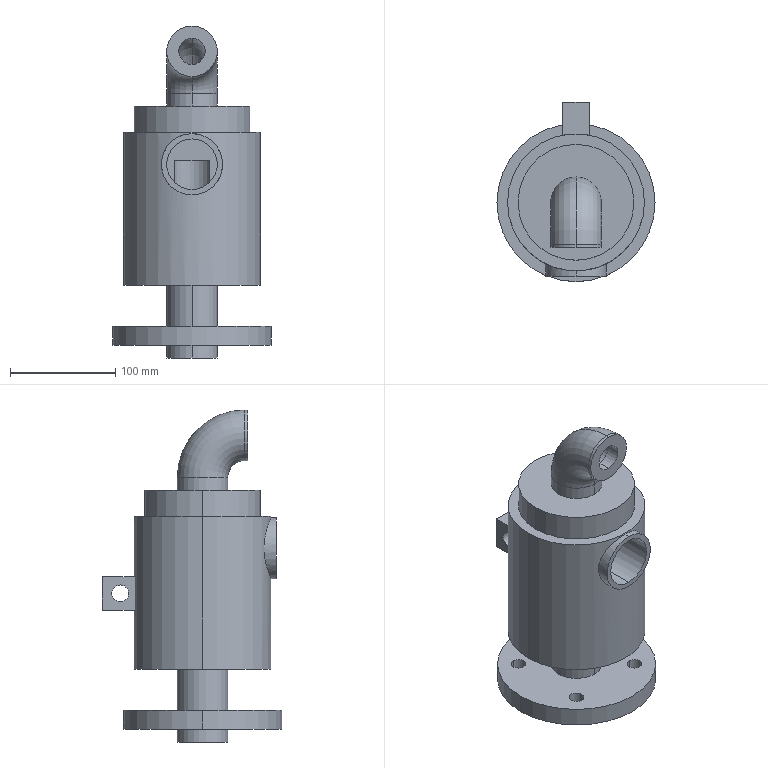Part | SolidWorks | features ICE 8, CirPattern 1, Extrusion 1, HoleWzd 1, Sweep 1, SweepCut 1 | 1 solid | 54 faces | box 150 x 170 x 315 mm | volume 2389466 mm3 | cylinder 34 | plane 16 | torus 4 | commonest cylinder face diameters 48 x10 14 x8 25 x4 16 x2 38 x2 58 x2